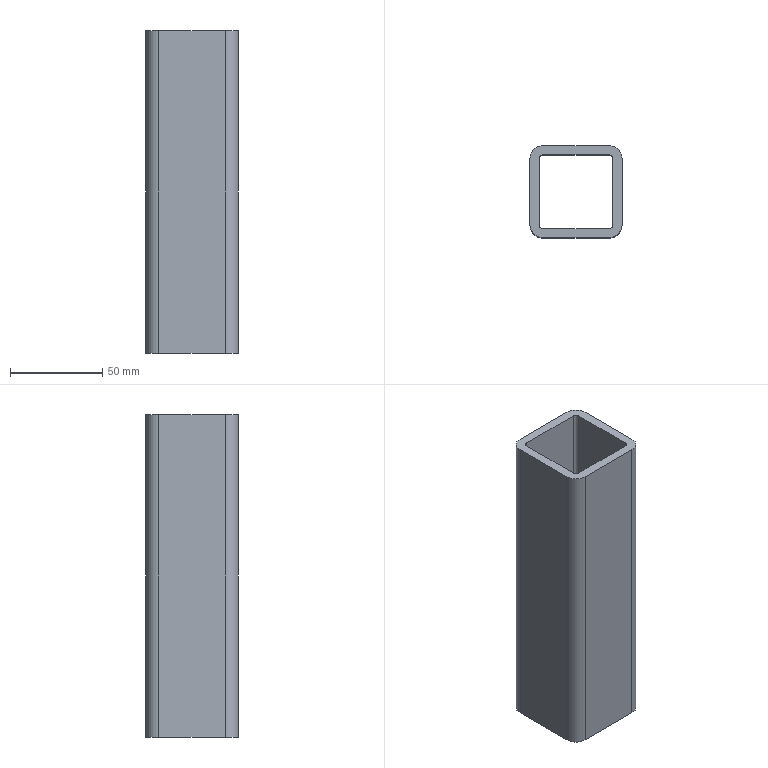Part | NX | 1 solid | 18 faces | box 50 x 50 x 175 mm | volume 150740 mm3 | plane 10 | cylinder 8 | commonest cylinder face diameters 4 x4 14 x4
STEP:
#1=CARTESIAN_POINT('',(-300.,874.,550.));
#2=VERTEX_POINT('',#1);
#3=CARTESIAN_POINT('',(-307.,881.,550.));
#4=VERTEX_POINT('',#3);
#5=CARTESIAN_POINT('',(-307.,874.,550.));
#6=DIRECTION('',(0.,0.,1.));
#7=DIRECTION('',(0.,-1.,0.));
#8=AXIS2_PLACEMENT_3D('',#5,#6,#7);
#9=CIRCLE('',#8,7.);
#10=EDGE_CURVE('',#2,#4,#9,.T.);
#11=ORIENTED_EDGE('',*,*,#10,.F.);
#12=CARTESIAN_POINT('',(-300.,874.,375.));
#13=VERTEX_POINT('',#12);
#14=CARTESIAN_POINT('',(-300.,874.,575.));
#15=DIRECTION('',(0.,0.,-1.));
#16=VECTOR('',#15,1000.);
#17=LINE('',#14,#16);
#18=EDGE_CURVE('',#2,#13,#17,.T.);
#19=ORIENTED_EDGE('',*,*,#18,.T.);
#20=CARTESIAN_POINT('',(-307.,881.,375.));
#21=VERTEX_POINT('',#20);
#22=CARTESIAN_POINT('',(-307.,874.,375.));
#23=DIRECTION('',(0.,0.,-1.));
#24=DIRECTION('',(0.,1.,0.));
#25=AXIS2_PLACEMENT_3D('',#22,#23,#24);
#26=CIRCLE('',#25,7.);
#27=EDGE_CURVE('',#21,#13,#26,.T.);
#28=ORIENTED_EDGE('',*,*,#27,.F.);
#29=CARTESIAN_POINT('',(-307.,881.,575.));
#30=DIRECTION('',(0.,0.,-1.));
#31=VECTOR('',#30,1000.);
#32=LINE('',#29,#31);
#33=EDGE_CURVE('',#4,#21,#32,.T.);
#34=ORIENTED_EDGE('',*,*,#33,.F.);
#35=EDGE_LOOP('',(#11,#19,#28,#34));
#36=FACE_BOUND('',#35,.T.);
#37=CARTESIAN_POINT('',(-307.,874.,575.));
#38=DIRECTION('',(0.,0.,-1.));
#39=DIRECTION('',(-1.,0.,0.));
#40=AXIS2_PLACEMENT_3D('',#37,#38,#39);
#41=CYLINDRICAL_SURFACE('',#40,7.);
#42=ADVANCED_FACE('',(#36),#41,.T.);
#43=CARTESIAN_POINT('',(-343.,881.,550.));
#44=VERTEX_POINT('',#43);
#45=CARTESIAN_POINT('',(-307.,881.,550.));
#46=DIRECTION('',(-1.,0.,0.));
#47=VECTOR('',#46,1000.);
#48=LINE('',#45,#47);
#49=EDGE_CURVE('',#4,#44,#48,.T.);
#50=ORIENTED_EDGE('',*,*,#49,.F.);
#51=ORIENTED_EDGE('',*,*,#33,.T.);
#52=CARTESIAN_POINT('',(-343.,881.,375.));
#53=VERTEX_POINT('',#52);
#54=CARTESIAN_POINT('',(-975.,881.,375.));
#55=DIRECTION('',(1.,0.,0.));
#56=VECTOR('',#55,1000.);
#57=LINE('',#54,#56);
#58=EDGE_CURVE('',#53,#21,#57,.T.);
#59=ORIENTED_EDGE('',*,*,#58,.F.);
#60=CARTESIAN_POINT('',(-343.,881.,575.));
#61=DIRECTION('',(0.,0.,-1.));
#62=VECTOR('',#61,1000.);
#63=LINE('',#60,#62);
#64=EDGE_CURVE('',#44,#53,#63,.T.);
#65=ORIENTED_EDGE('',*,*,#64,.F.);
#66=EDGE_LOOP('',(#50,#51,#59,#65));
#67=FACE_BOUND('',#66,.T.);
#68=CARTESIAN_POINT('',(-307.,881.,575.));
#69=DIRECTION('',(0.,-1.,0.));
#70=DIRECTION('',(1.,0.,0.));
#71=AXIS2_PLACEMENT_3D('',#68,#69,#70);
#72=PLANE('',#71);
#73=ADVANCED_FACE('',(#67),#72,.F.);
#74=CARTESIAN_POINT('',(-350.,874.,550.));
#75=VERTEX_POINT('',#74);
#76=CARTESIAN_POINT('',(-343.,874.,550.));
#77=DIRECTION('',(0.,0.,1.));
#78=DIRECTION('',(0.,-1.,0.));
#79=AXIS2_PLACEMENT_3D('',#76,#77,#78);
#80=CIRCLE('',#79,7.);
#81=EDGE_CURVE('',#44,#75,#80,.T.);
#82=ORIENTED_EDGE('',*,*,#81,.F.);
#83=ORIENTED_EDGE('',*,*,#64,.T.);
#84=CARTESIAN_POINT('',(-350.,874.,375.));
#85=VERTEX_POINT('',#84);
#86=CARTESIAN_POINT('',(-343.,874.,375.));
#87=DIRECTION('',(0.,0.,-1.));
#88=DIRECTION('',(0.,1.,0.));
#89=AXIS2_PLACEMENT_3D('',#86,#87,#88);
#90=CIRCLE('',#89,7.);
#91=EDGE_CURVE('',#85,#53,#90,.T.);
#92=ORIENTED_EDGE('',*,*,#91,.F.);
#93=CARTESIAN_POINT('',(-350.,874.,575.));
#94=DIRECTION('',(0.,0.,-1.));
#95=VECTOR('',#94,1000.);
#96=LINE('',#93,#95);
#97=EDGE_CURVE('',#75,#85,#96,.T.);
#98=ORIENTED_EDGE('',*,*,#97,.F.);
#99=EDGE_LOOP('',(#82,#83,#92,#98));
#100=FACE_BOUND('',#99,.T.);
#101=CARTESIAN_POINT('',(-343.,874.,575.));
#102=DIRECTION('',(0.,0.,-1.));
#103=DIRECTION('',(-1.,0.,0.));
#104=AXIS2_PLACEMENT_3D('',#101,#102,#103);
#105=CYLINDRICAL_SURFACE('',#104,7.);
#106=ADVANCED_FACE('',(#100),#105,.T.);
#107=CARTESIAN_POINT('',(-350.,838.,550.));
#108=VERTEX_POINT('',#107);
#109=CARTESIAN_POINT('',(-350.,0.,550.));
#110=DIRECTION('',(0.,1.,0.));
#111=VECTOR('',#110,1000.);
#112=LINE('',#109,#111);
#113=EDGE_CURVE('',#108,#75,#112,.T.);
#114=ORIENTED_EDGE('',*,*,#113,.T.);
#115=ORIENTED_EDGE('',*,*,#97,.T.);
#116=CARTESIAN_POINT('',(-350.,838.,375.));
#117=VERTEX_POINT('',#116);
#118=CARTESIAN_POINT('',(-350.,838.,375.));
#119=DIRECTION('',(0.,1.,0.));
#120=VECTOR('',#119,1000.);
#121=LINE('',#118,#120);
#122=EDGE_CURVE('',#117,#85,#121,.T.);
#123=ORIENTED_EDGE('',*,*,#122,.F.);
#124=CARTESIAN_POINT('',(-350.,838.,575.));
#125=DIRECTION('',(0.,0.,-1.));
#126=VECTOR('',#125,1000.);
#127=LINE('',#124,#126);
#128=EDGE_CURVE('',#108,#117,#127,.T.);
#129=ORIENTED_EDGE('',*,*,#128,.F.);
#130=EDGE_LOOP('',(#114,#115,#123,#129));
#131=FACE_BOUND('',#130,.T.);
#132=CARTESIAN_POINT('',(-350.,838.,575.));
#133=DIRECTION('',(1.,0.,0.));
#134=DIRECTION('',(0.,1.,0.));
#135=AXIS2_PLACEMENT_3D('',#132,#133,#134);
#136=PLANE('',#135);
#137=ADVANCED_FACE('',(#131),#136,.F.);
#138=CARTESIAN_POINT('',(-343.,831.,550.));
#139=VERTEX_POINT('',#138);
#140=CARTESIAN_POINT('',(-343.,838.,550.));
#141=DIRECTION('',(0.,0.,1.));
#142=DIRECTION('',(0.,-1.,0.));
#143=AXIS2_PLACEMENT_3D('',#140,#141,#142);
#144=CIRCLE('',#143,7.);
#145=EDGE_CURVE('',#108,#139,#144,.T.);
#146=ORIENTED_EDGE('',*,*,#145,.F.);
#147=ORIENTED_EDGE('',*,*,#128,.T.);
#148=CARTESIAN_POINT('',(-343.,831.,375.));
#149=VERTEX_POINT('',#148);
#150=CARTESIAN_POINT('',(-343.,838.,375.));
#151=DIRECTION('',(0.,0.,-1.));
#152=DIRECTION('',(0.,1.,0.));
#153=AXIS2_PLACEMENT_3D('',#150,#151,#152);
#154=CIRCLE('',#153,7.);
#155=EDGE_CURVE('',#149,#117,#154,.T.);
#156=ORIENTED_EDGE('',*,*,#155,.F.);
#157=CARTESIAN_POINT('',(-343.,831.,575.));
#158=DIRECTION('',(0.,0.,-1.));
#159=VECTOR('',#158,1000.);
#160=LINE('',#157,#159);
#161=EDGE_CURVE('',#139,#149,#160,.T.);
#162=ORIENTED_EDGE('',*,*,#161,.F.);
#163=EDGE_LOOP('',(#146,#147,#156,#162));
#164=FACE_BOUND('',#163,.T.);
#165=CARTESIAN_POINT('',(-343.,838.,575.));
#166=DIRECTION('',(0.,0.,-1.));
#167=DIRECTION('',(-1.,0.,0.));
#168=AXIS2_PLACEMENT_3D('',#165,#166,#167);
#169=CYLINDRICAL_SURFACE('',#168,7.);
#170=ADVANCED_FACE('',(#164),#169,.T.);
#171=CARTESIAN_POINT('',(-307.,831.,550.));
#172=VERTEX_POINT('',#171);
#173=CARTESIAN_POINT('',(-343.,831.,550.));
#174=DIRECTION('',(1.,0.,0.));
#175=VECTOR('',#174,1000.);
#176=LINE('',#173,#175);
#177=EDGE_CURVE('',#139,#172,#176,.T.);
#178=ORIENTED_EDGE('',*,*,#177,.F.);
#179=ORIENTED_EDGE('',*,*,#161,.T.);
#180=CARTESIAN_POINT('',(-307.,831.,375.));
#181=VERTEX_POINT('',#180);
#182=CARTESIAN_POINT('',(-975.,831.,375.));
#183=DIRECTION('',(1.,0.,0.));
#184=VECTOR('',#183,1000.);
#185=LINE('',#182,#184);
#186=EDGE_CURVE('',#149,#181,#185,.T.);
#187=ORIENTED_EDGE('',*,*,#186,.T.);
#188=CARTESIAN_POINT('',(-307.,831.,575.));
#189=DIRECTION('',(0.,0.,-1.));
#190=VECTOR('',#189,1000.);
#191=LINE('',#188,#190);
#192=EDGE_CURVE('',#172,#181,#191,.T.);
#193=ORIENTED_EDGE('',*,*,#192,.F.);
#194=EDGE_LOOP('',(#178,#179,#187,#193));
#195=FACE_BOUND('',#194,.T.);
#196=CARTESIAN_POINT('',(-343.,831.,575.));
#197=DIRECTION('',(0.,1.,0.));
#198=DIRECTION('',(-1.,0.,0.));
#199=AXIS2_PLACEMENT_3D('',#196,#197,#198);
#200=PLANE('',#199);
#201=ADVANCED_FACE('',(#195),#200,.F.);
#202=CARTESIAN_POINT('',(-300.,838.,550.));
#203=VERTEX_POINT('',#202);
#204=CARTESIAN_POINT('',(-307.,838.,550.));
#205=DIRECTION('',(0.,0.,1.));
#206=DIRECTION('',(0.,-1.,0.));
#207=AXIS2_PLACEMENT_3D('',#204,#205,#206);
#208=CIRCLE('',#207,7.);
#209=EDGE_CURVE('',#172,#203,#208,.T.);
#210=ORIENTED_EDGE('',*,*,#209,.F.);
#211=ORIENTED_EDGE('',*,*,#192,.T.);
#212=CARTESIAN_POINT('',(-300.,838.,375.));
#213=VERTEX_POINT('',#212);
#214=CARTESIAN_POINT('',(-307.,838.,375.));
#215=DIRECTION('',(0.,0.,-1.));
#216=DIRECTION('',(0.,1.,0.));
#217=AXIS2_PLACEMENT_3D('',#214,#215,#216);
#218=CIRCLE('',#217,7.);
#219=EDGE_CURVE('',#213,#181,#218,.T.);
#220=ORIENTED_EDGE('',*,*,#219,.F.);
#221=CARTESIAN_POINT('',(-300.,838.,575.));
#222=DIRECTION('',(0.,0.,-1.));
#223=VECTOR('',#222,1000.);
#224=LINE('',#221,#223);
#225=EDGE_CURVE('',#203,#213,#224,.T.);
#226=ORIENTED_EDGE('',*,*,#225,.F.);
#227=EDGE_LOOP('',(#210,#211,#220,#226));
#228=FACE_BOUND('',#227,.T.);
#229=CARTESIAN_POINT('',(-307.,838.,575.));
#230=DIRECTION('',(0.,0.,-1.));
#231=DIRECTION('',(-1.,0.,0.));
#232=AXIS2_PLACEMENT_3D('',#229,#230,#231);
#233=CYLINDRICAL_SURFACE('',#232,7.);
#234=ADVANCED_FACE('',(#228),#233,.T.);
#235=CARTESIAN_POINT('',(-343.,876.,550.));
#236=VERTEX_POINT('',#235);
#237=CARTESIAN_POINT('',(-343.,876.,375.));
#238=VERTEX_POINT('',#237);
#239=CARTESIAN_POINT('',(-343.,876.,575.));
#240=DIRECTION('',(0.,0.,-1.));
#241=VECTOR('',#240,1000.);
#242=LINE('',#239,#241);
#243=EDGE_CURVE('',#236,#238,#242,.T.);
#244=ORIENTED_EDGE('',*,*,#243,.F.);
#245=CARTESIAN_POINT('',(-345.,874.,550.));
#246=VERTEX_POINT('',#245);
#247=CARTESIAN_POINT('',(-343.,874.,550.));
#248=DIRECTION('',(0.,0.,1.));
#249=DIRECTION('',(0.,-1.,0.));
#250=AXIS2_PLACEMENT_3D('',#247,#248,#249);
#251=CIRCLE('',#250,2.);
#252=EDGE_CURVE('',#236,#246,#251,.T.);
#253=ORIENTED_EDGE('',*,*,#252,.T.);
#254=CARTESIAN_POINT('',(-345.,874.,375.));
#255=VERTEX_POINT('',#254);
#256=CARTESIAN_POINT('',(-345.,874.,575.));
#257=DIRECTION('',(0.,0.,-1.));
#258=VECTOR('',#257,1000.);
#259=LINE('',#256,#258);
#260=EDGE_CURVE('',#246,#255,#259,.T.);
#261=ORIENTED_EDGE('',*,*,#260,.T.);
#262=CARTESIAN_POINT('',(-343.,874.,375.));
#263=DIRECTION('',(0.,0.,-1.));
#264=DIRECTION('',(0.,1.,0.));
#265=AXIS2_PLACEMENT_3D('',#262,#263,#264);
#266=CIRCLE('',#265,2.);
#267=EDGE_CURVE('',#255,#238,#266,.T.);
#268=ORIENTED_EDGE('',*,*,#267,.T.);
#269=EDGE_LOOP('',(#244,#253,#261,#268));
#270=FACE_BOUND('',#269,.T.);
#271=CARTESIAN_POINT('',(-343.,874.,575.));
#272=DIRECTION('',(0.,0.,-1.));
#273=DIRECTION('',(-1.,0.,0.));
#274=AXIS2_PLACEMENT_3D('',#271,#272,#273);
#275=CYLINDRICAL_SURFACE('',#274,2.);
#276=ADVANCED_FACE('',(#270),#275,.F.);
#277=CARTESIAN_POINT('',(-307.,876.,550.));
#278=VERTEX_POINT('',#277);
#279=CARTESIAN_POINT('',(-307.,876.,375.));
#280=VERTEX_POINT('',#279);
#281=CARTESIAN_POINT('',(-307.,876.,575.));
#282=DIRECTION('',(0.,0.,-1.));
#283=VECTOR('',#282,1000.);
#284=LINE('',#281,#283);
#285=EDGE_CURVE('',#278,#280,#284,.T.);
#286=ORIENTED_EDGE('',*,*,#285,.F.);
#287=CARTESIAN_POINT('',(-307.,876.,550.));
#288=DIRECTION('',(-1.,0.,0.));
#289=VECTOR('',#288,1000.);
#290=LINE('',#287,#289);
#291=EDGE_CURVE('',#278,#236,#290,.T.);
#292=ORIENTED_EDGE('',*,*,#291,.T.);
#293=ORIENTED_EDGE('',*,*,#243,.T.);
#294=CARTESIAN_POINT('',(-307.,876.,375.));
#295=DIRECTION('',(1.,0.,0.));
#296=VECTOR('',#295,1000.);
#297=LINE('',#294,#296);
#298=EDGE_CURVE('',#238,#280,#297,.T.);
#299=ORIENTED_EDGE('',*,*,#298,.T.);
#300=EDGE_LOOP('',(#286,#292,#293,#299));
#301=FACE_BOUND('',#300,.T.);
#302=CARTESIAN_POINT('',(-307.,876.,575.));
#303=DIRECTION('',(0.,-1.,0.));
#304=DIRECTION('',(1.,0.,0.));
#305=AXIS2_PLACEMENT_3D('',#302,#303,#304);
#306=PLANE('',#305);
#307=ADVANCED_FACE('',(#301),#306,.T.);
#308=CARTESIAN_POINT('',(-305.,874.,550.));
#309=VERTEX_POINT('',#308);
#310=CARTESIAN_POINT('',(-305.,874.,375.));
#311=VERTEX_POINT('',#310);
#312=CARTESIAN_POINT('',(-305.,874.,575.));
#313=DIRECTION('',(0.,0.,-1.));
#314=VECTOR('',#313,1000.);
#315=LINE('',#312,#314);
#316=EDGE_CURVE('',#309,#311,#315,.T.);
#317=ORIENTED_EDGE('',*,*,#316,.F.);
#318=CARTESIAN_POINT('',(-307.,874.,550.));
#319=DIRECTION('',(0.,0.,1.));
#320=DIRECTION('',(0.,-1.,0.));
#321=AXIS2_PLACEMENT_3D('',#318,#319,#320);
#322=CIRCLE('',#321,2.);
#323=EDGE_CURVE('',#309,#278,#322,.T.);
#324=ORIENTED_EDGE('',*,*,#323,.T.);
#325=ORIENTED_EDGE('',*,*,#285,.T.);
#326=CARTESIAN_POINT('',(-307.,874.,375.));
#327=DIRECTION('',(0.,0.,-1.));
#328=DIRECTION('',(0.,1.,0.));
#329=AXIS2_PLACEMENT_3D('',#326,#327,#328);
#330=CIRCLE('',#329,2.);
#331=EDGE_CURVE('',#280,#311,#330,.T.);
#332=ORIENTED_EDGE('',*,*,#331,.T.);
#333=EDGE_LOOP('',(#317,#324,#325,#332));
#334=FACE_BOUND('',#333,.T.);
#335=CARTESIAN_POINT('',(-307.,874.,575.));
#336=DIRECTION('',(0.,0.,-1.));
#337=DIRECTION('',(-1.,0.,0.));
#338=AXIS2_PLACEMENT_3D('',#335,#336,#337);
#339=CYLINDRICAL_SURFACE('',#338,2.);
#340=ADVANCED_FACE('',(#334),#339,.F.);
#341=CARTESIAN_POINT('',(-305.,838.,550.));
#342=VERTEX_POINT('',#341);
#343=CARTESIAN_POINT('',(-305.,838.,375.));
#344=VERTEX_POINT('',#343);
#345=CARTESIAN_POINT('',(-305.,838.,575.));
#346=DIRECTION('',(0.,0.,-1.));
#347=VECTOR('',#346,1000.);
#348=LINE('',#345,#347);
#349=EDGE_CURVE('',#342,#344,#348,.T.);
#350=ORIENTED_EDGE('',*,*,#349,.F.);
#351=CARTESIAN_POINT('',(-305.,874.,550.));
#352=DIRECTION('',(0.,1.,0.));
#353=VECTOR('',#352,1000.);
#354=LINE('',#351,#353);
#355=EDGE_CURVE('',#342,#309,#354,.T.);
#356=ORIENTED_EDGE('',*,*,#355,.T.);
#357=ORIENTED_EDGE('',*,*,#316,.T.);
#358=CARTESIAN_POINT('',(-305.,874.,375.));
#359=DIRECTION('',(0.,-1.,0.));
#360=VECTOR('',#359,1000.);
#361=LINE('',#358,#360);
#362=EDGE_CURVE('',#311,#344,#361,.T.);
#363=ORIENTED_EDGE('',*,*,#362,.T.);
#364=EDGE_LOOP('',(#350,#356,#357,#363));
#365=FACE_BOUND('',#364,.T.);
#366=CARTESIAN_POINT('',(-305.,874.,575.));
#367=DIRECTION('',(-1.,0.,0.));
#368=DIRECTION('',(0.,-1.,0.));
#369=AXIS2_PLACEMENT_3D('',#366,#367,#368);
#370=PLANE('',#369);
#371=ADVANCED_FACE('',(#365),#370,.T.);
#372=CARTESIAN_POINT('',(-307.,836.,550.));
#373=VERTEX_POINT('',#372);
#374=CARTESIAN_POINT('',(-307.,836.,375.));
#375=VERTEX_POINT('',#374);
#376=CARTESIAN_POINT('',(-307.,836.,575.));
#377=DIRECTION('',(0.,0.,-1.));
#378=VECTOR('',#377,1000.);
#379=LINE('',#376,#378);
#380=EDGE_CURVE('',#373,#375,#379,.T.);
#381=ORIENTED_EDGE('',*,*,#380,.F.);
#382=CARTESIAN_POINT('',(-307.,838.,550.));
#383=DIRECTION('',(0.,0.,1.));
#384=DIRECTION('',(0.,-1.,0.));
#385=AXIS2_PLACEMENT_3D('',#382,#383,#384);
#386=CIRCLE('',#385,2.);
#387=EDGE_CURVE('',#373,#342,#386,.T.);
#388=ORIENTED_EDGE('',*,*,#387,.T.);
#389=ORIENTED_EDGE('',*,*,#349,.T.);
#390=CARTESIAN_POINT('',(-307.,838.,375.));
#391=DIRECTION('',(0.,0.,-1.));
#392=DIRECTION('',(0.,1.,0.));
#393=AXIS2_PLACEMENT_3D('',#390,#391,#392);
#394=CIRCLE('',#393,2.);
#395=EDGE_CURVE('',#344,#375,#394,.T.);
#396=ORIENTED_EDGE('',*,*,#395,.T.);
#397=EDGE_LOOP('',(#381,#388,#389,#396));
#398=FACE_BOUND('',#397,.T.);
#399=CARTESIAN_POINT('',(-307.,838.,575.));
#400=DIRECTION('',(0.,0.,-1.));
#401=DIRECTION('',(-1.,0.,0.));
#402=AXIS2_PLACEMENT_3D('',#399,#400,#401);
#403=CYLINDRICAL_SURFACE('',#402,2.);
#404=ADVANCED_FACE('',(#398),#403,.F.);
#405=CARTESIAN_POINT('',(-343.,836.,550.));
#406=VERTEX_POINT('',#405);
#407=CARTESIAN_POINT('',(-343.,836.,375.));
#408=VERTEX_POINT('',#407);
#409=CARTESIAN_POINT('',(-343.,836.,575.));
#410=DIRECTION('',(0.,0.,-1.));
#411=VECTOR('',#410,1000.);
#412=LINE('',#409,#411);
#413=EDGE_CURVE('',#406,#408,#412,.T.);
#414=ORIENTED_EDGE('',*,*,#413,.F.);
#415=CARTESIAN_POINT('',(-343.,836.,550.));
#416=DIRECTION('',(1.,0.,0.));
#417=VECTOR('',#416,1000.);
#418=LINE('',#415,#417);
#419=EDGE_CURVE('',#406,#373,#418,.T.);
#420=ORIENTED_EDGE('',*,*,#419,.T.);
#421=ORIENTED_EDGE('',*,*,#380,.T.);
#422=CARTESIAN_POINT('',(-343.,836.,375.));
#423=DIRECTION('',(-1.,0.,0.));
#424=VECTOR('',#423,1000.);
#425=LINE('',#422,#424);
#426=EDGE_CURVE('',#375,#408,#425,.T.);
#427=ORIENTED_EDGE('',*,*,#426,.T.);
#428=EDGE_LOOP('',(#414,#420,#421,#427));
#429=FACE_BOUND('',#428,.T.);
#430=CARTESIAN_POINT('',(-343.,836.,575.));
#431=DIRECTION('',(0.,1.,0.));
#432=DIRECTION('',(-1.,0.,0.));
#433=AXIS2_PLACEMENT_3D('',#430,#431,#432);
#434=PLANE('',#433);
#435=ADVANCED_FACE('',(#429),#434,.T.);
#436=CARTESIAN_POINT('',(-345.,838.,550.));
#437=VERTEX_POINT('',#436);
#438=CARTESIAN_POINT('',(-345.,838.,375.));
#439=VERTEX_POINT('',#438);
#440=CARTESIAN_POINT('',(-345.,838.,575.));
#441=DIRECTION('',(0.,0.,-1.));
#442=VECTOR('',#441,1000.);
#443=LINE('',#440,#442);
#444=EDGE_CURVE('',#437,#439,#443,.T.);
#445=ORIENTED_EDGE('',*,*,#444,.F.);
#446=CARTESIAN_POINT('',(-343.,838.,550.));
#447=DIRECTION('',(0.,0.,1.));
#448=DIRECTION('',(0.,-1.,0.));
#449=AXIS2_PLACEMENT_3D('',#446,#447,#448);
#450=CIRCLE('',#449,2.);
#451=EDGE_CURVE('',#437,#406,#450,.T.);
#452=ORIENTED_EDGE('',*,*,#451,.T.);
#453=ORIENTED_EDGE('',*,*,#413,.T.);
#454=CARTESIAN_POINT('',(-343.,838.,375.));
#455=DIRECTION('',(0.,0.,-1.));
#456=DIRECTION('',(0.,1.,0.));
#457=AXIS2_PLACEMENT_3D('',#454,#455,#456);
#458=CIRCLE('',#457,2.);
#459=EDGE_CURVE('',#408,#439,#458,.T.);
#460=ORIENTED_EDGE('',*,*,#459,.T.);
#461=EDGE_LOOP('',(#445,#452,#453,#460));
#462=FACE_BOUND('',#461,.T.);
#463=CARTESIAN_POINT('',(-343.,838.,575.));
#464=DIRECTION('',(0.,0.,-1.));
#465=DIRECTION('',(-1.,0.,0.));
#466=AXIS2_PLACEMENT_3D('',#463,#464,#465);
#467=CYLINDRICAL_SURFACE('',#466,2.);
#468=ADVANCED_FACE('',(#462),#467,.F.);
#469=ORIENTED_EDGE('',*,*,#260,.F.);
#470=CARTESIAN_POINT('',(-345.,838.,550.));
#471=DIRECTION('',(0.,-1.,0.));
#472=VECTOR('',#471,1000.);
#473=LINE('',#470,#472);
#474=EDGE_CURVE('',#246,#437,#473,.T.);
#475=ORIENTED_EDGE('',*,*,#474,.T.);
#476=ORIENTED_EDGE('',*,*,#444,.T.);
#477=CARTESIAN_POINT('',(-345.,838.,375.));
#478=DIRECTION('',(0.,1.,0.));
#479=VECTOR('',#478,1000.);
#480=LINE('',#477,#479);
#481=EDGE_CURVE('',#439,#255,#480,.T.);
#482=ORIENTED_EDGE('',*,*,#481,.T.);
#483=EDGE_LOOP('',(#469,#475,#476,#482));
#484=FACE_BOUND('',#483,.T.);
#485=CARTESIAN_POINT('',(-345.,838.,575.));
#486=DIRECTION('',(1.,0.,0.));
#487=DIRECTION('',(0.,1.,0.));
#488=AXIS2_PLACEMENT_3D('',#485,#486,#487);
#489=PLANE('',#488);
#490=ADVANCED_FACE('',(#484),#489,.T.);
#491=CARTESIAN_POINT('',(-300.,874.,550.));
#492=DIRECTION('',(0.,1.,0.));
#493=VECTOR('',#492,1000.);
#494=LINE('',#491,#493);
#495=EDGE_CURVE('',#203,#2,#494,.T.);
#496=ORIENTED_EDGE('',*,*,#495,.F.);
#497=ORIENTED_EDGE('',*,*,#225,.T.);
#498=CARTESIAN_POINT('',(-300.,874.,375.));
#499=DIRECTION('',(0.,-1.,0.));
#500=VECTOR('',#499,1000.);
#501=LINE('',#498,#500);
#502=EDGE_CURVE('',#13,#213,#501,.T.);
#503=ORIENTED_EDGE('',*,*,#502,.F.);
#504=ORIENTED_EDGE('',*,*,#18,.F.);
#505=EDGE_LOOP('',(#496,#497,#503,#504));
#506=FACE_BOUND('',#505,.T.);
#507=CARTESIAN_POINT('',(-300.,874.,575.));
#508=DIRECTION('',(-1.,0.,0.));
#509=DIRECTION('',(0.,-1.,0.));
#510=AXIS2_PLACEMENT_3D('',#507,#508,#509);
#511=PLANE('',#510);
#512=ADVANCED_FACE('',(#506),#511,.F.);
#513=ORIENTED_EDGE('',*,*,#481,.F.);
#514=ORIENTED_EDGE('',*,*,#459,.F.);
#515=ORIENTED_EDGE('',*,*,#426,.F.);
#516=ORIENTED_EDGE('',*,*,#395,.F.);
#517=ORIENTED_EDGE('',*,*,#362,.F.);
#518=ORIENTED_EDGE('',*,*,#331,.F.);
#519=ORIENTED_EDGE('',*,*,#298,.F.);
#520=ORIENTED_EDGE('',*,*,#267,.F.);
#521=EDGE_LOOP('',(#513,#514,#515,#516,#517,#518,#519,#520));
#522=FACE_BOUND('',#521,.T.);
#523=ORIENTED_EDGE('',*,*,#91,.T.);
#524=ORIENTED_EDGE('',*,*,#58,.T.);
#525=ORIENTED_EDGE('',*,*,#27,.T.);
#526=ORIENTED_EDGE('',*,*,#502,.T.);
#527=ORIENTED_EDGE('',*,*,#219,.T.);
#528=ORIENTED_EDGE('',*,*,#186,.F.);
#529=ORIENTED_EDGE('',*,*,#155,.T.);
#530=ORIENTED_EDGE('',*,*,#122,.T.);
#531=EDGE_LOOP('',(#523,#524,#525,#526,#527,#528,#529,#530));
#532=FACE_BOUND('',#531,.T.);
#533=CARTESIAN_POINT('',(-975.,874.,375.));
#534=DIRECTION('',(0.,0.,-1.));
#535=DIRECTION('',(0.,1.,0.));
#536=AXIS2_PLACEMENT_3D('',#533,#534,#535);
#537=PLANE('',#536);
#538=ADVANCED_FACE('',(#522,#532),#537,.T.);
#539=ORIENTED_EDGE('',*,*,#291,.F.);
#540=ORIENTED_EDGE('',*,*,#323,.F.);
#541=ORIENTED_EDGE('',*,*,#355,.F.);
#542=ORIENTED_EDGE('',*,*,#387,.F.);
#543=ORIENTED_EDGE('',*,*,#419,.F.);
#544=ORIENTED_EDGE('',*,*,#451,.F.);
#545=ORIENTED_EDGE('',*,*,#474,.F.);
#546=ORIENTED_EDGE('',*,*,#252,.F.);
#547=EDGE_LOOP('',(#539,#540,#541,#542,#543,#544,#545,#546));
#548=FACE_BOUND('',#547,.T.);
#549=ORIENTED_EDGE('',*,*,#10,.T.);
#550=ORIENTED_EDGE('',*,*,#49,.T.);
#551=ORIENTED_EDGE('',*,*,#81,.T.);
#552=ORIENTED_EDGE('',*,*,#113,.F.);
#553=ORIENTED_EDGE('',*,*,#145,.T.);
#554=ORIENTED_EDGE('',*,*,#177,.T.);
#555=ORIENTED_EDGE('',*,*,#209,.T.);
#556=ORIENTED_EDGE('',*,*,#495,.T.);
#557=EDGE_LOOP('',(#549,#550,#551,#552,#553,#554,#555,#556));
#558=FACE_BOUND('',#557,.T.);
#559=CARTESIAN_POINT('',(-343.,0.,550.));
#560=DIRECTION('',(0.,0.,1.));
#561=DIRECTION('',(0.,-1.,0.));
#562=AXIS2_PLACEMENT_3D('',#559,#560,#561);
#563=PLANE('',#562);
#564=ADVANCED_FACE('',(#548,#558),#563,.T.);
#565=CLOSED_SHELL('',(#42,#73,#106,#137,#170,#201,#234,#276,#307,#340,#371,#404,#435,#468,#490,#512,#538,#564));
#566=MANIFOLD_SOLID_BREP('',#565);
#567=(LENGTH_UNIT()NAMED_UNIT(*)SI_UNIT(.MILLI.,.METRE.));
#568=UNCERTAINTY_MEASURE_WITH_UNIT(LENGTH_MEASURE(0.00001),#567,'','');
#569=(NAMED_UNIT(*)PLANE_ANGLE_UNIT()SI_UNIT($,.RADIAN.));
#570=(NAMED_UNIT(*)SI_UNIT($,.STERADIAN.)SOLID_ANGLE_UNIT());
#571=(GEOMETRIC_REPRESENTATION_CONTEXT(3)GLOBAL_UNCERTAINTY_ASSIGNED_CONTEXT((#568))GLOBAL_UNIT_ASSIGNED_CONTEXT((#567,#569,#570))REPRESENTATION_CONTEXT('',''));
#572=ADVANCED_BREP_SHAPE_REPRESENTATION('',(#566),#571);